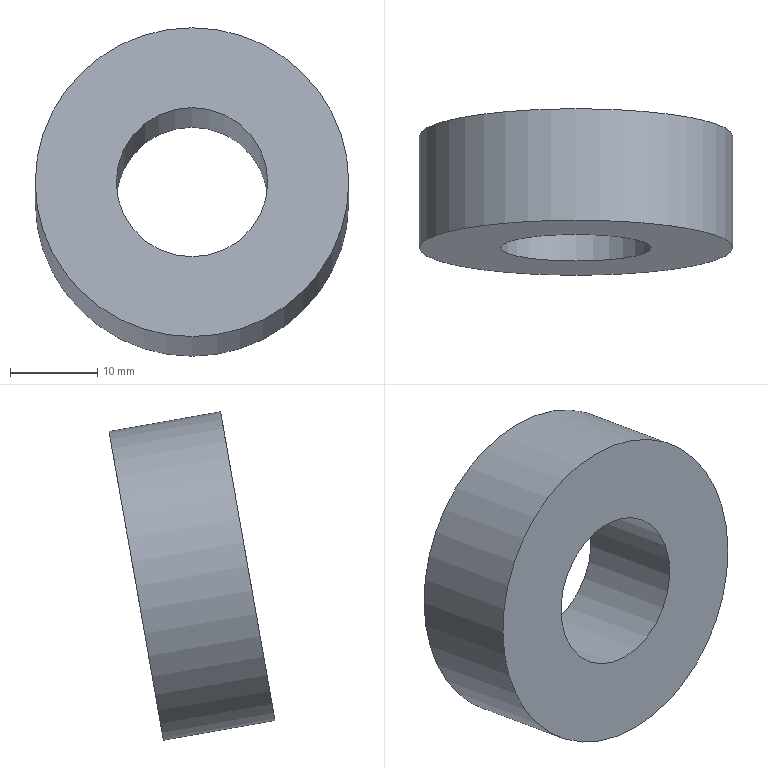Part | NX | features solid 2 | 1 solid | 4 faces | box 36 x 19.054 x 37.711 mm | volume 10141 mm3 | cylinder 2 | plane 2 | commonest cylinder face diameters 17.4 x1 36 x1
STEP:
#1=CARTESIAN_POINT('',(767.8,-797.53,12.214));
#2=VERTEX_POINT('',#1);
#3=CARTESIAN_POINT('',(776.5,-797.53,12.214));
#4=DIRECTION('',(0.,-0.9848,0.1736));
#5=DIRECTION('',(-1.,0.,0.));
#6=AXIS2_PLACEMENT_3D('',#3,#4,#5);
#7=CIRCLE('',#6,8.7);
#8=EDGE_CURVE('',#2,#2,#7,.T.);
#9=ORIENTED_EDGE('',*,*,#8,.T.);
#10=EDGE_LOOP('',(#9));
#11=FACE_BOUND('',#10,.T.);
#12=CARTESIAN_POINT('',(767.8,-784.728,9.956));
#13=VERTEX_POINT('',#12);
#14=CARTESIAN_POINT('',(776.5,-784.728,9.956));
#15=DIRECTION('',(0.,-0.9848,0.1736));
#16=DIRECTION('',(-1.,0.,0.));
#17=AXIS2_PLACEMENT_3D('',#14,#15,#16);
#18=CIRCLE('',#17,8.7);
#19=EDGE_CURVE('',#13,#13,#18,.T.);
#20=ORIENTED_EDGE('',*,*,#19,.F.);
#21=EDGE_LOOP('',(#20));
#22=FACE_BOUND('',#21,.T.);
#23=CARTESIAN_POINT('',(776.5,-797.53,12.214));
#24=DIRECTION('',(0.,0.9848,-0.1736));
#25=DIRECTION('',(1.,0.,0.));
#26=AXIS2_PLACEMENT_3D('',#23,#24,#25);
#27=CYLINDRICAL_SURFACE('',#26,8.7);
#28=ADVANCED_FACE('',(#11,#22),#27,.F.);
#29=CARTESIAN_POINT('',(758.5,-797.53,12.214));
#30=VERTEX_POINT('',#29);
#31=CARTESIAN_POINT('',(776.5,-797.53,12.214));
#32=DIRECTION('',(0.,-0.9848,0.1736));
#33=DIRECTION('',(-1.,0.,0.));
#34=AXIS2_PLACEMENT_3D('',#31,#32,#33);
#35=CIRCLE('',#34,18.);
#36=EDGE_CURVE('',#30,#30,#35,.T.);
#37=ORIENTED_EDGE('',*,*,#36,.F.);
#38=EDGE_LOOP('',(#37));
#39=FACE_BOUND('',#38,.T.);
#40=CARTESIAN_POINT('',(758.5,-784.728,9.956));
#41=VERTEX_POINT('',#40);
#42=CARTESIAN_POINT('',(776.5,-784.728,9.956));
#43=DIRECTION('',(0.,-0.9848,0.1736));
#44=DIRECTION('',(-1.,0.,0.));
#45=AXIS2_PLACEMENT_3D('',#42,#43,#44);
#46=CIRCLE('',#45,18.);
#47=EDGE_CURVE('',#41,#41,#46,.T.);
#48=ORIENTED_EDGE('',*,*,#47,.T.);
#49=EDGE_LOOP('',(#48));
#50=FACE_BOUND('',#49,.T.);
#51=CARTESIAN_POINT('',(776.5,-797.53,12.214));
#52=DIRECTION('',(0.,0.9848,-0.1736));
#53=DIRECTION('',(1.,0.,0.));
#54=AXIS2_PLACEMENT_3D('',#51,#52,#53);
#55=CYLINDRICAL_SURFACE('',#54,18.);
#56=ADVANCED_FACE('',(#39,#50),#55,.T.);
#57=ORIENTED_EDGE('',*,*,#8,.F.);
#58=EDGE_LOOP('',(#57));
#59=FACE_BOUND('',#58,.T.);
#60=ORIENTED_EDGE('',*,*,#36,.T.);
#61=EDGE_LOOP('',(#60));
#62=FACE_BOUND('',#61,.T.);
#63=CARTESIAN_POINT('',(776.5,-797.53,12.214));
#64=DIRECTION('',(0.,-0.9848,0.1736));
#65=DIRECTION('',(-1.,0.,0.));
#66=AXIS2_PLACEMENT_3D('',#63,#64,#65);
#67=PLANE('',#66);
#68=ADVANCED_FACE('',(#59,#62),#67,.T.);
#69=ORIENTED_EDGE('',*,*,#19,.T.);
#70=EDGE_LOOP('',(#69));
#71=FACE_BOUND('',#70,.T.);
#72=ORIENTED_EDGE('',*,*,#47,.F.);
#73=EDGE_LOOP('',(#72));
#74=FACE_BOUND('',#73,.T.);
#75=CARTESIAN_POINT('',(776.5,-784.728,9.956));
#76=DIRECTION('',(0.,-0.9848,0.1736));
#77=DIRECTION('',(-1.,0.,0.));
#78=AXIS2_PLACEMENT_3D('',#75,#76,#77);
#79=PLANE('',#78);
#80=ADVANCED_FACE('',(#71,#74),#79,.F.);
#81=CLOSED_SHELL('',(#28,#56,#68,#80));
#82=MANIFOLD_SOLID_BREP('',#81);
#83=(LENGTH_UNIT()NAMED_UNIT(*)SI_UNIT(.MILLI.,.METRE.));
#84=UNCERTAINTY_MEASURE_WITH_UNIT(LENGTH_MEASURE(0.00001),#83,'','');
#85=(NAMED_UNIT(*)PLANE_ANGLE_UNIT()SI_UNIT($,.RADIAN.));
#86=(NAMED_UNIT(*)SI_UNIT($,.STERADIAN.)SOLID_ANGLE_UNIT());
#87=(GEOMETRIC_REPRESENTATION_CONTEXT(3)GLOBAL_UNCERTAINTY_ASSIGNED_CONTEXT((#84))GLOBAL_UNIT_ASSIGNED_CONTEXT((#83,#85,#86))REPRESENTATION_CONTEXT('',''));
#88=ADVANCED_BREP_SHAPE_REPRESENTATION('',(#82),#87);